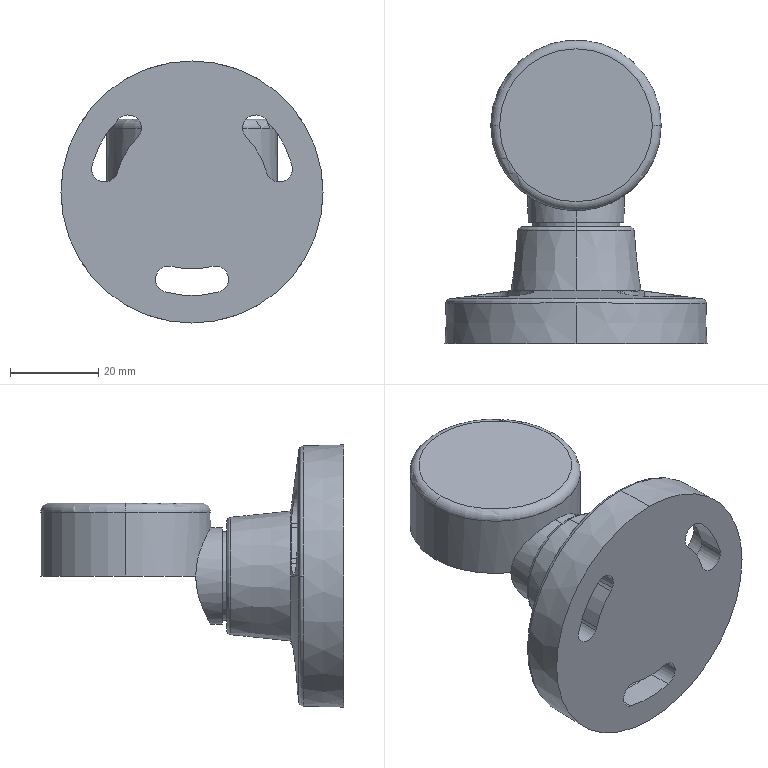Part | SolidWorks | features ICE 7, Fillet 2, CirPattern 1, Extrusion 1, RevCut 1 | 1 solid | 63 faces | box 59.5 x 68.85 x 59.5 mm | volume 56089 mm3 | cylinder 43 | plane 8 | torus 6 | cone 6 | commonest cylinder face diameters 6 x12 10 x12 31 x3 35 x3 38.7 x3 47 x3